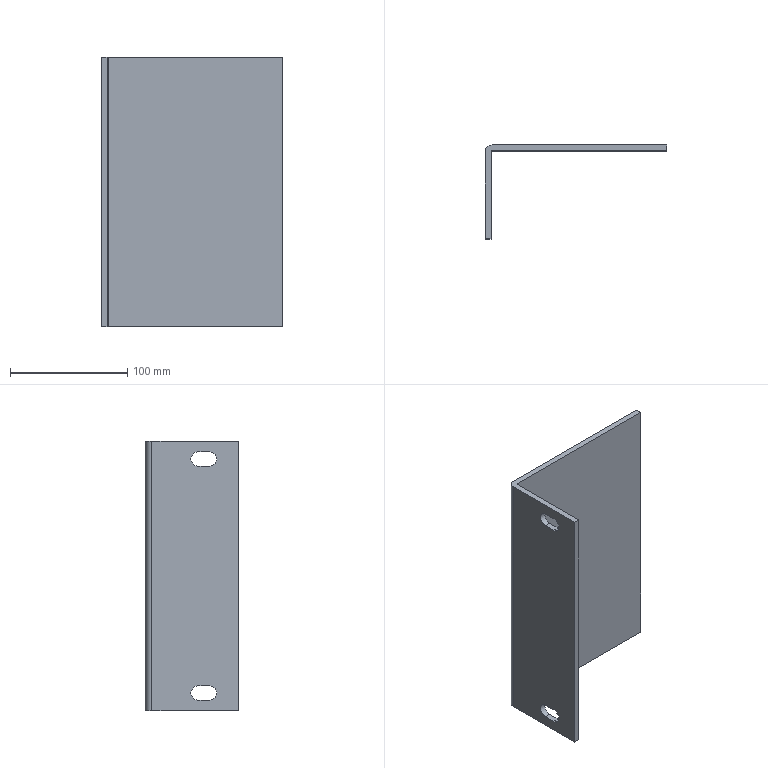Part | STEP file | PN_0002_support angle steel | 1 solid | 20 faces | box 155 x 80 x 230 mm | volume 260571 mm3 | plane 12 | cylinder 8 | commonest cylinder face diameters 12 x6 1.473 x1 11.473 x1